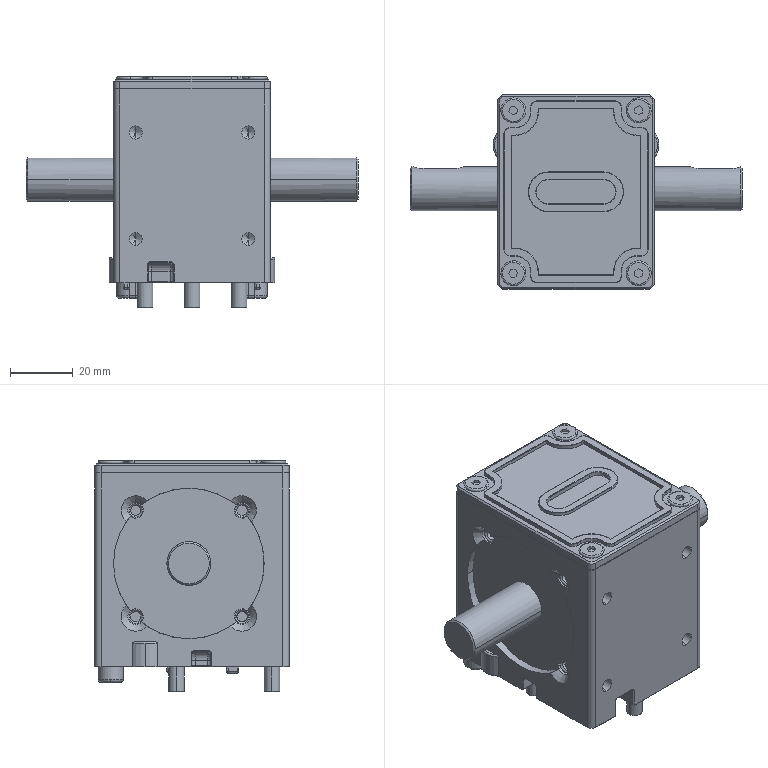Part | SolidWorks | features BaseBody 13, ICE 5, Chamfer 3 | 12 solids | 1016 faces | box 106 x 62 x 74 mm | volume 204451 mm3 | plane 451 | cylinder 310 | cone 179 | torus 56 | sphere 12 | spline 8 | commonest cylinder face diameters 2 x51 5 x36 1 x24 4 x24 0.2 x18 0.6 x16